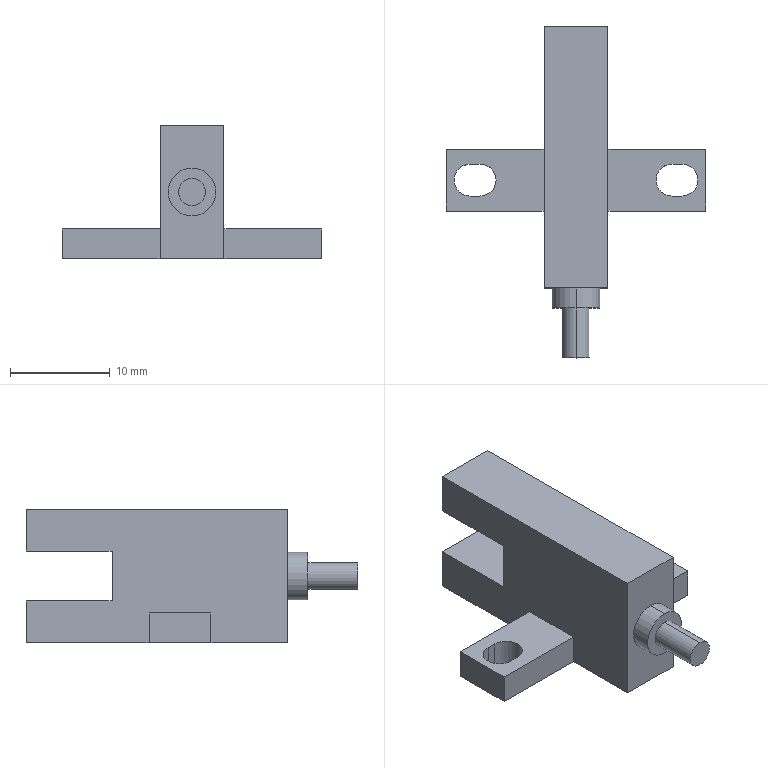Part | STEP file | 复件 aaPT-T44^复件 FFH85-PL-M75-B3-01_三轴模组 | 1 solid | 34 faces | box 26 x 33.2 x 13.4 mm | volume 2334 mm3 | plane 24 | cylinder 10 | commonest cylinder face diameters 3.2 x6 2.7 x2 4.8 x2
STEP:
#1=CARTESIAN_POINT('',(0.,-15.1,9.1));
#2=VERTEX_POINT('',#1);
#3=CARTESIAN_POINT('',(0.,-15.1,4.3));
#4=VERTEX_POINT('',#3);
#5=CARTESIAN_POINT('',(0.,-15.1,6.7));
#6=DIRECTION('',(0.,1.,0.));
#7=DIRECTION('',(0.,0.,1.));
#8=AXIS2_PLACEMENT_3D('',#5,#6,#7);
#9=CIRCLE('',#8,2.4);
#10=EDGE_CURVE('',#2,#4,#9,.T.);
#11=ORIENTED_EDGE('',*,*,#10,.T.);
#12=CARTESIAN_POINT('',(0.,-13.1,4.3));
#13=VERTEX_POINT('',#12);
#14=CARTESIAN_POINT('',(0.,-15.1,4.3));
#15=DIRECTION('',(0.,1.,0.));
#16=VECTOR('',#15,1000.);
#17=LINE('',#14,#16);
#18=EDGE_CURVE('',#4,#13,#17,.T.);
#19=ORIENTED_EDGE('',*,*,#18,.T.);
#20=CARTESIAN_POINT('',(0.,-13.1,9.1));
#21=VERTEX_POINT('',#20);
#22=CARTESIAN_POINT('',(0.,-13.1,6.7));
#23=DIRECTION('',(0.,-1.,0.));
#24=DIRECTION('',(0.,0.,1.));
#25=AXIS2_PLACEMENT_3D('',#22,#23,#24);
#26=CIRCLE('',#25,2.4);
#27=EDGE_CURVE('',#13,#21,#26,.T.);
#28=ORIENTED_EDGE('',*,*,#27,.T.);
#29=CARTESIAN_POINT('',(0.,-15.1,9.1));
#30=DIRECTION('',(0.,1.,0.));
#31=VECTOR('',#30,1000.);
#32=LINE('',#29,#31);
#33=EDGE_CURVE('',#2,#21,#32,.T.);
#34=ORIENTED_EDGE('',*,*,#33,.F.);
#35=EDGE_LOOP('',(#11,#19,#28,#34));
#36=FACE_OUTER_BOUND('',#35,.T.);
#37=CARTESIAN_POINT('',(0.,-15.1,6.7));
#38=DIRECTION('',(0.,1.,0.));
#39=DIRECTION('',(0.,0.,1.));
#40=AXIS2_PLACEMENT_3D('',#37,#38,#39);
#41=CYLINDRICAL_SURFACE('',#40,2.4);
#42=ADVANCED_FACE('',(#36),#41,.T.);
#43=CARTESIAN_POINT('',(12.2,-2.3,0.));
#44=VERTEX_POINT('',#43);
#45=CARTESIAN_POINT('',(10.575,-0.7002,0.));
#46=VERTEX_POINT('',#45);
#47=CARTESIAN_POINT('',(10.6,-2.3,0.));
#48=DIRECTION('',(0.,0.,1.));
#49=DIRECTION('',(1.,0.,0.));
#50=AXIS2_PLACEMENT_3D('',#47,#48,#49);
#51=CIRCLE('',#50,1.6);
#52=EDGE_CURVE('',#44,#46,#51,.T.);
#53=ORIENTED_EDGE('',*,*,#52,.F.);
#54=CARTESIAN_POINT('',(12.2,-2.3,3.));
#55=VERTEX_POINT('',#54);
#56=CARTESIAN_POINT('',(12.2,-2.3,0.));
#57=DIRECTION('',(0.,0.,1.));
#58=VECTOR('',#57,1000.);
#59=LINE('',#56,#58);
#60=EDGE_CURVE('',#44,#55,#59,.T.);
#61=ORIENTED_EDGE('',*,*,#60,.T.);
#62=CARTESIAN_POINT('',(10.575,-0.7002,3.));
#63=VERTEX_POINT('',#62);
#64=CARTESIAN_POINT('',(10.6,-2.3,3.));
#65=DIRECTION('',(0.,0.,1.));
#66=DIRECTION('',(1.,0.,0.));
#67=AXIS2_PLACEMENT_3D('',#64,#65,#66);
#68=CIRCLE('',#67,1.6);
#69=EDGE_CURVE('',#55,#63,#68,.T.);
#70=ORIENTED_EDGE('',*,*,#69,.T.);
#71=CARTESIAN_POINT('',(10.575,-0.7002,0.));
#72=DIRECTION('',(0.,0.,1.));
#73=VECTOR('',#72,1000.);
#74=LINE('',#71,#73);
#75=EDGE_CURVE('',#46,#63,#74,.T.);
#76=ORIENTED_EDGE('',*,*,#75,.F.);
#77=EDGE_LOOP('',(#53,#61,#70,#76));
#78=FACE_OUTER_BOUND('',#77,.T.);
#79=CARTESIAN_POINT('',(10.6,-2.3,0.));
#80=DIRECTION('',(0.,0.,1.));
#81=DIRECTION('',(1.,0.,0.));
#82=AXIS2_PLACEMENT_3D('',#79,#80,#81);
#83=CYLINDRICAL_SURFACE('',#82,1.6);
#84=ADVANCED_FACE('',(#78),#83,.F.);
#85=CARTESIAN_POINT('',(-8.,-2.3,0.));
#86=VERTEX_POINT('',#85);
#87=CARTESIAN_POINT('',(-9.6,-0.7002,0.));
#88=VERTEX_POINT('',#87);
#89=CARTESIAN_POINT('',(-9.6,-2.3,0.));
#90=DIRECTION('',(0.,0.,1.));
#91=DIRECTION('',(1.,0.,0.));
#92=AXIS2_PLACEMENT_3D('',#89,#90,#91);
#93=CIRCLE('',#92,1.6);
#94=EDGE_CURVE('',#86,#88,#93,.T.);
#95=ORIENTED_EDGE('',*,*,#94,.F.);
#96=CARTESIAN_POINT('',(-8.,-2.3,3.));
#97=VERTEX_POINT('',#96);
#98=CARTESIAN_POINT('',(-8.,-2.3,0.));
#99=DIRECTION('',(0.,0.,1.));
#100=VECTOR('',#99,1000.);
#101=LINE('',#98,#100);
#102=EDGE_CURVE('',#86,#97,#101,.T.);
#103=ORIENTED_EDGE('',*,*,#102,.T.);
#104=CARTESIAN_POINT('',(-9.6,-0.7002,3.));
#105=VERTEX_POINT('',#104);
#106=CARTESIAN_POINT('',(-9.6,-2.3,3.));
#107=DIRECTION('',(0.,0.,-1.));
#108=DIRECTION('',(1.,0.,0.));
#109=AXIS2_PLACEMENT_3D('',#106,#107,#108);
#110=CIRCLE('',#109,1.6);
#111=EDGE_CURVE('',#105,#97,#110,.T.);
#112=ORIENTED_EDGE('',*,*,#111,.F.);
#113=CARTESIAN_POINT('',(-9.6,-0.7002,0.));
#114=DIRECTION('',(0.,0.,1.));
#115=VECTOR('',#114,1000.);
#116=LINE('',#113,#115);
#117=EDGE_CURVE('',#88,#105,#116,.T.);
#118=ORIENTED_EDGE('',*,*,#117,.F.);
#119=EDGE_LOOP('',(#95,#103,#112,#118));
#120=FACE_OUTER_BOUND('',#119,.T.);
#121=CARTESIAN_POINT('',(-9.6,-2.3,0.));
#122=DIRECTION('',(0.,0.,1.));
#123=DIRECTION('',(1.,0.,0.));
#124=AXIS2_PLACEMENT_3D('',#121,#122,#123);
#125=CYLINDRICAL_SURFACE('',#124,1.6);
#126=ADVANCED_FACE('',(#120),#125,.F.);
#127=CARTESIAN_POINT('',(0.,-20.1,8.05));
#128=VERTEX_POINT('',#127);
#129=CARTESIAN_POINT('',(0.,-20.1,5.35));
#130=VERTEX_POINT('',#129);
#131=CARTESIAN_POINT('',(0.,-20.1,6.7));
#132=DIRECTION('',(0.,1.,0.));
#133=DIRECTION('',(0.,0.,1.));
#134=AXIS2_PLACEMENT_3D('',#131,#132,#133);
#135=CIRCLE('',#134,1.35);
#136=EDGE_CURVE('',#128,#130,#135,.T.);
#137=ORIENTED_EDGE('',*,*,#136,.T.);
#138=CARTESIAN_POINT('',(0.,-15.1,5.35));
#139=VERTEX_POINT('',#138);
#140=CARTESIAN_POINT('',(0.,-20.1,5.35));
#141=DIRECTION('',(0.,1.,0.));
#142=VECTOR('',#141,1000.);
#143=LINE('',#140,#142);
#144=EDGE_CURVE('',#130,#139,#143,.T.);
#145=ORIENTED_EDGE('',*,*,#144,.T.);
#146=CARTESIAN_POINT('',(0.,-15.1,8.05));
#147=VERTEX_POINT('',#146);
#148=CARTESIAN_POINT('',(0.,-15.1,6.7));
#149=DIRECTION('',(0.,1.,0.));
#150=DIRECTION('',(0.,0.,1.));
#151=AXIS2_PLACEMENT_3D('',#148,#149,#150);
#152=CIRCLE('',#151,1.35);
#153=EDGE_CURVE('',#147,#139,#152,.T.);
#154=ORIENTED_EDGE('',*,*,#153,.F.);
#155=CARTESIAN_POINT('',(0.,-20.1,8.05));
#156=DIRECTION('',(0.,1.,0.));
#157=VECTOR('',#156,1000.);
#158=LINE('',#155,#157);
#159=EDGE_CURVE('',#128,#147,#158,.T.);
#160=ORIENTED_EDGE('',*,*,#159,.F.);
#161=EDGE_LOOP('',(#137,#145,#154,#160));
#162=FACE_OUTER_BOUND('',#161,.T.);
#163=CARTESIAN_POINT('',(0.,-20.1,6.7));
#164=DIRECTION('',(0.,1.,0.));
#165=DIRECTION('',(0.,0.,1.));
#166=AXIS2_PLACEMENT_3D('',#163,#164,#165);
#167=CYLINDRICAL_SURFACE('',#166,1.35);
#168=ADVANCED_FACE('',(#162),#167,.T.);
#169=CARTESIAN_POINT('',(3.2,-13.1,0.));
#170=VERTEX_POINT('',#169);
#171=CARTESIAN_POINT('',(3.2,-13.1,13.4));
#172=VERTEX_POINT('',#171);
#173=CARTESIAN_POINT('',(3.2,-13.1,13.4));
#174=DIRECTION('',(0.,0.,1.));
#175=VECTOR('',#174,1000.);
#176=LINE('',#173,#175);
#177=EDGE_CURVE('',#170,#172,#176,.T.);
#178=ORIENTED_EDGE('',*,*,#177,.F.);
#179=CARTESIAN_POINT('',(3.2,-5.4,0.));
#180=VERTEX_POINT('',#179);
#181=CARTESIAN_POINT('',(3.2,-13.1,0.));
#182=DIRECTION('',(0.,-1.,0.));
#183=VECTOR('',#182,1000.);
#184=LINE('',#181,#183);
#185=EDGE_CURVE('',#180,#170,#184,.T.);
#186=ORIENTED_EDGE('',*,*,#185,.F.);
#187=CARTESIAN_POINT('',(3.2,-5.4,3.));
#188=VERTEX_POINT('',#187);
#189=CARTESIAN_POINT('',(3.2,-5.4,13.4));
#190=DIRECTION('',(0.,0.,-1.));
#191=VECTOR('',#190,1000.);
#192=LINE('',#189,#191);
#193=EDGE_CURVE('',#188,#180,#192,.T.);
#194=ORIENTED_EDGE('',*,*,#193,.F.);
#195=CARTESIAN_POINT('',(3.2,0.8,3.));
#196=VERTEX_POINT('',#195);
#197=CARTESIAN_POINT('',(3.2,-13.1,3.));
#198=DIRECTION('',(0.,-1.,0.));
#199=VECTOR('',#198,1000.);
#200=LINE('',#197,#199);
#201=EDGE_CURVE('',#196,#188,#200,.T.);
#202=ORIENTED_EDGE('',*,*,#201,.F.);
#203=CARTESIAN_POINT('',(3.2,0.8,0.));
#204=VERTEX_POINT('',#203);
#205=CARTESIAN_POINT('',(3.2,0.8,13.4));
#206=DIRECTION('',(0.,0.,1.));
#207=VECTOR('',#206,1000.);
#208=LINE('',#205,#207);
#209=EDGE_CURVE('',#204,#196,#208,.T.);
#210=ORIENTED_EDGE('',*,*,#209,.F.);
#211=CARTESIAN_POINT('',(3.2,13.1,0.));
#212=VERTEX_POINT('',#211);
#213=CARTESIAN_POINT('',(3.2,-13.1,0.));
#214=DIRECTION('',(0.,-1.,0.));
#215=VECTOR('',#214,1000.);
#216=LINE('',#213,#215);
#217=EDGE_CURVE('',#212,#204,#216,.T.);
#218=ORIENTED_EDGE('',*,*,#217,.F.);
#219=CARTESIAN_POINT('',(3.2,13.1,4.2));
#220=VERTEX_POINT('',#219);
#221=CARTESIAN_POINT('',(3.2,13.1,13.4));
#222=DIRECTION('',(0.,0.,-1.));
#223=VECTOR('',#222,1000.);
#224=LINE('',#221,#223);
#225=EDGE_CURVE('',#220,#212,#224,.T.);
#226=ORIENTED_EDGE('',*,*,#225,.F.);
#227=CARTESIAN_POINT('',(3.2,4.5,4.2));
#228=VERTEX_POINT('',#227);
#229=CARTESIAN_POINT('',(3.2,-13.1,4.2));
#230=DIRECTION('',(0.,1.,0.));
#231=VECTOR('',#230,1000.);
#232=LINE('',#229,#231);
#233=EDGE_CURVE('',#228,#220,#232,.T.);
#234=ORIENTED_EDGE('',*,*,#233,.F.);
#235=CARTESIAN_POINT('',(3.2,4.5,9.2));
#236=VERTEX_POINT('',#235);
#237=CARTESIAN_POINT('',(3.2,4.5,13.4));
#238=DIRECTION('',(0.,0.,-1.));
#239=VECTOR('',#238,1000.);
#240=LINE('',#237,#239);
#241=EDGE_CURVE('',#236,#228,#240,.T.);
#242=ORIENTED_EDGE('',*,*,#241,.F.);
#243=CARTESIAN_POINT('',(3.2,13.1,9.2));
#244=VERTEX_POINT('',#243);
#245=CARTESIAN_POINT('',(3.2,-13.1,9.2));
#246=DIRECTION('',(0.,-1.,0.));
#247=VECTOR('',#246,1000.);
#248=LINE('',#245,#247);
#249=EDGE_CURVE('',#244,#236,#248,.T.);
#250=ORIENTED_EDGE('',*,*,#249,.F.);
#251=CARTESIAN_POINT('',(3.2,13.1,13.4));
#252=VERTEX_POINT('',#251);
#253=CARTESIAN_POINT('',(3.2,13.1,13.4));
#254=DIRECTION('',(0.,0.,-1.));
#255=VECTOR('',#254,1000.);
#256=LINE('',#253,#255);
#257=EDGE_CURVE('',#252,#244,#256,.T.);
#258=ORIENTED_EDGE('',*,*,#257,.F.);
#259=CARTESIAN_POINT('',(3.2,-13.1,13.4));
#260=DIRECTION('',(0.,1.,0.));
#261=VECTOR('',#260,1000.);
#262=LINE('',#259,#261);
#263=EDGE_CURVE('',#172,#252,#262,.T.);
#264=ORIENTED_EDGE('',*,*,#263,.F.);
#265=EDGE_LOOP('',(#178,#186,#194,#202,#210,#218,#226,#234,#242,#250,#258,#264));
#266=FACE_OUTER_BOUND('',#265,.T.);
#267=CARTESIAN_POINT('',(3.2,-13.1,13.4));
#268=DIRECTION('',(-1.,0.,0.));
#269=DIRECTION('',(0.,0.,1.));
#270=AXIS2_PLACEMENT_3D('',#267,#268,#269);
#271=PLANE('',#270);
#272=ADVANCED_FACE('',(#266),#271,.F.);
#273=CARTESIAN_POINT('',(-3.2,13.1,13.4));
#274=VERTEX_POINT('',#273);
#275=CARTESIAN_POINT('',(13.,13.1,13.4));
#276=DIRECTION('',(1.,0.,0.));
#277=VECTOR('',#276,1000.);
#278=LINE('',#275,#277);
#279=EDGE_CURVE('',#274,#252,#278,.T.);
#280=ORIENTED_EDGE('',*,*,#279,.F.);
#281=CARTESIAN_POINT('',(-3.2,-13.1,13.4));
#282=VERTEX_POINT('',#281);
#283=CARTESIAN_POINT('',(-3.2,13.1,13.4));
#284=DIRECTION('',(0.,1.,0.));
#285=VECTOR('',#284,1000.);
#286=LINE('',#283,#285);
#287=EDGE_CURVE('',#282,#274,#286,.T.);
#288=ORIENTED_EDGE('',*,*,#287,.F.);
#289=CARTESIAN_POINT('',(13.,-13.1,13.4));
#290=DIRECTION('',(-1.,0.,0.));
#291=VECTOR('',#290,1000.);
#292=LINE('',#289,#291);
#293=EDGE_CURVE('',#172,#282,#292,.T.);
#294=ORIENTED_EDGE('',*,*,#293,.F.);
#295=ORIENTED_EDGE('',*,*,#263,.T.);
#296=EDGE_LOOP('',(#280,#288,#294,#295));
#297=FACE_OUTER_BOUND('',#296,.T.);
#298=CARTESIAN_POINT('',(13.,13.1,13.4));
#299=DIRECTION('',(0.,0.,-1.));
#300=DIRECTION('',(-1.,0.,0.));
#301=AXIS2_PLACEMENT_3D('',#298,#299,#300);
#302=PLANE('',#301);
#303=ADVANCED_FACE('',(#297),#302,.F.);
#304=ORIENTED_EDGE('',*,*,#293,.T.);
#305=CARTESIAN_POINT('',(-3.2,-13.1,0.));
#306=VERTEX_POINT('',#305);
#307=CARTESIAN_POINT('',(-3.2,-13.1,13.4));
#308=DIRECTION('',(0.,0.,1.));
#309=VECTOR('',#308,1000.);
#310=LINE('',#307,#309);
#311=EDGE_CURVE('',#306,#282,#310,.T.);
#312=ORIENTED_EDGE('',*,*,#311,.F.);
#313=CARTESIAN_POINT('',(-13.,-13.1,0.));
#314=DIRECTION('',(-1.,0.,0.));
#315=VECTOR('',#314,1000.);
#316=LINE('',#313,#315);
#317=EDGE_CURVE('',#170,#306,#316,.T.);
#318=ORIENTED_EDGE('',*,*,#317,.F.);
#319=ORIENTED_EDGE('',*,*,#177,.T.);
#320=EDGE_LOOP('',(#304,#312,#318,#319));
#321=FACE_OUTER_BOUND('',#320,.T.);
#322=CARTESIAN_POINT('',(0.,-13.1,6.7));
#323=DIRECTION('',(0.,-1.,0.));
#324=DIRECTION('',(0.,0.,1.));
#325=AXIS2_PLACEMENT_3D('',#322,#323,#324);
#326=CIRCLE('',#325,2.4);
#327=EDGE_CURVE('',#21,#13,#326,.T.);
#328=ORIENTED_EDGE('',*,*,#327,.F.);
#329=ORIENTED_EDGE('',*,*,#27,.F.);
#330=EDGE_LOOP('',(#328,#329));
#331=FACE_BOUND('',#330,.T.);
#332=CARTESIAN_POINT('',(-13.,-13.1,13.4));
#333=DIRECTION('',(0.,1.,0.));
#334=DIRECTION('',(0.,0.,1.));
#335=AXIS2_PLACEMENT_3D('',#332,#333,#334);
#336=PLANE('',#335);
#337=ADVANCED_FACE('',(#321,#331),#336,.F.);
#338=CARTESIAN_POINT('',(10.6,-3.9,0.));
#339=VERTEX_POINT('',#338);
#340=CARTESIAN_POINT('',(10.6,-2.3,0.));
#341=DIRECTION('',(0.,0.,1.));
#342=DIRECTION('',(1.,0.,0.));
#343=AXIS2_PLACEMENT_3D('',#340,#341,#342);
#344=CIRCLE('',#343,1.6);
#345=EDGE_CURVE('',#339,#44,#344,.T.);
#346=ORIENTED_EDGE('',*,*,#345,.T.);
#347=ORIENTED_EDGE('',*,*,#52,.T.);
#348=CARTESIAN_POINT('',(9.6,-0.7002,0.));
#349=VERTEX_POINT('',#348);
#350=CARTESIAN_POINT('',(10.575,-0.7002,0.));
#351=DIRECTION('',(-1.,0.,0.));
#352=VECTOR('',#351,1000.);
#353=LINE('',#350,#352);
#354=EDGE_CURVE('',#46,#349,#353,.T.);
#355=ORIENTED_EDGE('',*,*,#354,.T.);
#356=CARTESIAN_POINT('',(9.625,-3.9,0.));
#357=VERTEX_POINT('',#356);
#358=CARTESIAN_POINT('',(9.6,-2.3,0.));
#359=DIRECTION('',(0.,0.,1.));
#360=DIRECTION('',(1.,0.,0.));
#361=AXIS2_PLACEMENT_3D('',#358,#359,#360);
#362=CIRCLE('',#361,1.6);
#363=EDGE_CURVE('',#349,#357,#362,.T.);
#364=ORIENTED_EDGE('',*,*,#363,.T.);
#365=CARTESIAN_POINT('',(10.6,-3.9,0.));
#366=DIRECTION('',(1.,0.,0.));
#367=VECTOR('',#366,1000.);
#368=LINE('',#365,#367);
#369=EDGE_CURVE('',#357,#339,#368,.T.);
#370=ORIENTED_EDGE('',*,*,#369,.T.);
#371=EDGE_LOOP('',(#346,#347,#355,#364,#370));
#372=FACE_BOUND('',#371,.T.);
#373=CARTESIAN_POINT('',(-9.625,-3.9,0.));
#374=VERTEX_POINT('',#373);
#375=CARTESIAN_POINT('',(-9.6,-2.3,0.));
#376=DIRECTION('',(0.,0.,1.));
#377=DIRECTION('',(1.,0.,0.));
#378=AXIS2_PLACEMENT_3D('',#375,#376,#377);
#379=CIRCLE('',#378,1.6);
#380=EDGE_CURVE('',#374,#86,#379,.T.);
#381=ORIENTED_EDGE('',*,*,#380,.T.);
#382=ORIENTED_EDGE('',*,*,#94,.T.);
#383=CARTESIAN_POINT('',(-10.575,-0.7002,0.));
#384=VERTEX_POINT('',#383);
#385=CARTESIAN_POINT('',(-10.575,-0.7002,0.));
#386=DIRECTION('',(-1.,0.,0.));
#387=VECTOR('',#386,1000.);
#388=LINE('',#385,#387);
#389=EDGE_CURVE('',#88,#384,#388,.T.);
#390=ORIENTED_EDGE('',*,*,#389,.T.);
#391=CARTESIAN_POINT('',(-10.6,-3.9,0.));
#392=VERTEX_POINT('',#391);
#393=CARTESIAN_POINT('',(-10.6,-2.3,0.));
#394=DIRECTION('',(0.,0.,1.));
#395=DIRECTION('',(1.,0.,0.));
#396=AXIS2_PLACEMENT_3D('',#393,#394,#395);
#397=CIRCLE('',#396,1.6);
#398=EDGE_CURVE('',#384,#392,#397,.T.);
#399=ORIENTED_EDGE('',*,*,#398,.T.);
#400=CARTESIAN_POINT('',(-10.6,-3.9,0.));
#401=DIRECTION('',(1.,0.,0.));
#402=VECTOR('',#401,1000.);
#403=LINE('',#400,#402);
#404=EDGE_CURVE('',#392,#374,#403,.T.);
#405=ORIENTED_EDGE('',*,*,#404,.T.);
#406=EDGE_LOOP('',(#381,#382,#390,#399,#405));
#407=FACE_BOUND('',#406,.T.);
#408=CARTESIAN_POINT('',(-13.,0.8,0.));
#409=VERTEX_POINT('',#408);
#410=CARTESIAN_POINT('',(-3.2,0.8,0.));
#411=VERTEX_POINT('',#410);
#412=CARTESIAN_POINT('',(13.,0.8,0.));
#413=DIRECTION('',(1.,0.,0.));
#414=VECTOR('',#413,1000.);
#415=LINE('',#412,#414);
#416=EDGE_CURVE('',#409,#411,#415,.T.);
#417=ORIENTED_EDGE('',*,*,#416,.T.);
#418=CARTESIAN_POINT('',(-3.2,13.1,0.));
#419=VERTEX_POINT('',#418);
#420=CARTESIAN_POINT('',(-3.2,13.1,0.));
#421=DIRECTION('',(0.,1.,0.));
#422=VECTOR('',#421,1000.);
#423=LINE('',#420,#422);
#424=EDGE_CURVE('',#411,#419,#423,.T.);
#425=ORIENTED_EDGE('',*,*,#424,.T.);
#426=CARTESIAN_POINT('',(13.,13.1,0.));
#427=DIRECTION('',(1.,0.,0.));
#428=VECTOR('',#427,1000.);
#429=LINE('',#426,#428);
#430=EDGE_CURVE('',#419,#212,#429,.T.);
#431=ORIENTED_EDGE('',*,*,#430,.T.);
#432=ORIENTED_EDGE('',*,*,#217,.T.);
#433=CARTESIAN_POINT('',(13.,0.8,0.));
#434=VERTEX_POINT('',#433);
#435=CARTESIAN_POINT('',(13.,0.8,0.));
#436=DIRECTION('',(1.,0.,0.));
#437=VECTOR('',#436,1000.);
#438=LINE('',#435,#437);
#439=EDGE_CURVE('',#204,#434,#438,.T.);
#440=ORIENTED_EDGE('',*,*,#439,.T.);
#441=CARTESIAN_POINT('',(13.,-5.4,0.));
#442=VERTEX_POINT('',#441);
#443=CARTESIAN_POINT('',(13.,13.1,0.));
#444=DIRECTION('',(0.,-1.,0.));
#445=VECTOR('',#444,1000.);
#446=LINE('',#443,#445);
#447=EDGE_CURVE('',#434,#442,#446,.T.);
#448=ORIENTED_EDGE('',*,*,#447,.T.);
#449=CARTESIAN_POINT('',(13.,-5.4,0.));
#450=DIRECTION('',(-1.,0.,0.));
#451=VECTOR('',#450,1000.);
#452=LINE('',#449,#451);
#453=EDGE_CURVE('',#442,#180,#452,.T.);
#454=ORIENTED_EDGE('',*,*,#453,.T.);
#455=ORIENTED_EDGE('',*,*,#185,.T.);
#456=ORIENTED_EDGE('',*,*,#317,.T.);
#457=CARTESIAN_POINT('',(-3.2,-5.4,0.));
#458=VERTEX_POINT('',#457);
#459=CARTESIAN_POINT('',(-3.2,13.1,0.));
#460=DIRECTION('',(0.,1.,0.));
#461=VECTOR('',#460,1000.);
#462=LINE('',#459,#461);
#463=EDGE_CURVE('',#306,#458,#462,.T.);
#464=ORIENTED_EDGE('',*,*,#463,.T.);
#465=CARTESIAN_POINT('',(-13.,-5.4,0.));
#466=VERTEX_POINT('',#465);
#467=CARTESIAN_POINT('',(13.,-5.4,0.));
#468=DIRECTION('',(-1.,0.,0.));
#469=VECTOR('',#468,1000.);
#470=LINE('',#467,#469);
#471=EDGE_CURVE('',#458,#466,#470,.T.);
#472=ORIENTED_EDGE('',*,*,#471,.T.);
#473=CARTESIAN_POINT('',(-13.,13.1,0.));
#474=DIRECTION('',(0.,1.,0.));
#475=VECTOR('',#474,1000.);
#476=LINE('',#473,#475);
#477=EDGE_CURVE('',#466,#409,#476,.T.);
#478=ORIENTED_EDGE('',*,*,#477,.T.);
#479=EDGE_LOOP('',(#417,#425,#431,#432,#440,#448,#454,#455,#456,#464,#472,#478));
#480=FACE_OUTER_BOUND('',#479,.T.);
#481=CARTESIAN_POINT('',(13.,13.1,0.));
#482=DIRECTION('',(0.,0.,-1.));
#483=DIRECTION('',(-1.,0.,0.));
#484=AXIS2_PLACEMENT_3D('',#481,#482,#483);
#485=PLANE('',#484);
#486=ADVANCED_FACE('',(#372,#407,#480),#485,.T.);
#487=ORIENTED_EDGE('',*,*,#453,.F.);
#488=CARTESIAN_POINT('',(13.,-5.4,3.));
#489=VERTEX_POINT('',#488);
#490=CARTESIAN_POINT('',(13.,-5.4,0.));
#491=DIRECTION('',(0.,0.,-1.));
#492=VECTOR('',#491,1000.);
#493=LINE('',#490,#492);
#494=EDGE_CURVE('',#489,#442,#493,.T.);
#495=ORIENTED_EDGE('',*,*,#494,.F.);
#496=CARTESIAN_POINT('',(13.,-5.4,3.));
#497=DIRECTION('',(1.,0.,0.));
#498=VECTOR('',#497,1000.);
#499=LINE('',#496,#498);
#500=EDGE_CURVE('',#188,#489,#499,.T.);
#501=ORIENTED_EDGE('',*,*,#500,.F.);
#502=ORIENTED_EDGE('',*,*,#193,.T.);
#503=EDGE_LOOP('',(#487,#495,#501,#502));
#504=FACE_OUTER_BOUND('',#503,.T.);
#505=CARTESIAN_POINT('',(13.,-5.4,0.));
#506=DIRECTION('',(0.,1.,0.));
#507=DIRECTION('',(0.,0.,1.));
#508=AXIS2_PLACEMENT_3D('',#505,#506,#507);
#509=PLANE('',#508);
#510=ADVANCED_FACE('',(#504),#509,.F.);
#511=CARTESIAN_POINT('',(10.6,-3.9,3.));
#512=VERTEX_POINT('',#511);
#513=CARTESIAN_POINT('',(9.625,-3.9,3.));
#514=VERTEX_POINT('',#513);
#515=CARTESIAN_POINT('',(10.6,-3.9,3.));
#516=DIRECTION('',(-1.,0.,0.));
#517=VECTOR('',#516,1000.);
#518=LINE('',#515,#517);
#519=EDGE_CURVE('',#512,#514,#518,.T.);
#520=ORIENTED_EDGE('',*,*,#519,.T.);
#521=CARTESIAN_POINT('',(9.6,-0.7002,3.));
#522=VERTEX_POINT('',#521);
#523=CARTESIAN_POINT('',(9.6,-2.3,3.));
#524=DIRECTION('',(0.,0.,1.));
#525=DIRECTION('',(1.,0.,0.));
#526=AXIS2_PLACEMENT_3D('',#523,#524,#525);
#527=CIRCLE('',#526,1.6);
#528=EDGE_CURVE('',#522,#514,#527,.T.);
#529=ORIENTED_EDGE('',*,*,#528,.F.);
#530=CARTESIAN_POINT('',(10.575,-0.7002,3.));
#531=DIRECTION('',(1.,0.,0.));
#532=VECTOR('',#531,1000.);
#533=LINE('',#530,#532);
#534=EDGE_CURVE('',#522,#63,#533,.T.);
#535=ORIENTED_EDGE('',*,*,#534,.T.);
#536=ORIENTED_EDGE('',*,*,#69,.F.);
#537=CARTESIAN_POINT('',(10.6,-2.3,3.));
#538=DIRECTION('',(0.,0.,1.));
#539=DIRECTION('',(1.,0.,0.));
#540=AXIS2_PLACEMENT_3D('',#537,#538,#539);
#541=CIRCLE('',#540,1.6);
#542=EDGE_CURVE('',#512,#55,#541,.T.);
#543=ORIENTED_EDGE('',*,*,#542,.F.);
#544=EDGE_LOOP('',(#520,#529,#535,#536,#543));
#545=FACE_BOUND('',#544,.T.);
#546=ORIENTED_EDGE('',*,*,#201,.T.);
#547=ORIENTED_EDGE('',*,*,#500,.T.);
#548=CARTESIAN_POINT('',(13.,0.8,3.));
#549=VERTEX_POINT('',#548);
#550=CARTESIAN_POINT('',(13.,-13.1,3.));
#551=DIRECTION('',(0.,-1.,0.));
#552=VECTOR('',#551,1000.);
#553=LINE('',#550,#552);
#554=EDGE_CURVE('',#549,#489,#553,.T.);
#555=ORIENTED_EDGE('',*,*,#554,.F.);
#556=CARTESIAN_POINT('',(13.,0.8,3.));
#557=DIRECTION('',(1.,0.,0.));
#558=VECTOR('',#557,1000.);
#559=LINE('',#556,#558);
#560=EDGE_CURVE('',#196,#549,#559,.T.);
#561=ORIENTED_EDGE('',*,*,#560,.F.);
#562=EDGE_LOOP('',(#546,#547,#555,#561));
#563=FACE_OUTER_BOUND('',#562,.T.);
#564=CARTESIAN_POINT('',(13.,-13.1,3.));
#565=DIRECTION('',(0.,0.,-1.));
#566=DIRECTION('',(-1.,0.,0.));
#567=AXIS2_PLACEMENT_3D('',#564,#565,#566);
#568=PLANE('',#567);
#569=ADVANCED_FACE('',(#545,#563),#568,.F.);
#570=ORIENTED_EDGE('',*,*,#439,.F.);
#571=ORIENTED_EDGE('',*,*,#209,.T.);
#572=ORIENTED_EDGE('',*,*,#560,.T.);
#573=CARTESIAN_POINT('',(13.,0.8,0.));
#574=DIRECTION('',(0.,0.,1.));
#575=VECTOR('',#574,1000.);
#576=LINE('',#573,#575);
#577=EDGE_CURVE('',#434,#549,#576,.T.);
#578=ORIENTED_EDGE('',*,*,#577,.F.);
#579=EDGE_LOOP('',(#570,#571,#572,#578));
#580=FACE_OUTER_BOUND('',#579,.T.);
#581=CARTESIAN_POINT('',(13.,0.8,0.));
#582=DIRECTION('',(0.,-1.,0.));
#583=DIRECTION('',(0.,0.,-1.));
#584=AXIS2_PLACEMENT_3D('',#581,#582,#583);
#585=PLANE('',#584);
#586=ADVANCED_FACE('',(#580),#585,.F.);
#587=CARTESIAN_POINT('',(-3.2,13.1,4.2));
#588=VERTEX_POINT('',#587);
#589=CARTESIAN_POINT('',(-3.2,13.1,13.4));
#590=DIRECTION('',(0.,0.,-1.));
#591=VECTOR('',#590,1000.);
#592=LINE('',#589,#591);
#593=EDGE_CURVE('',#588,#419,#592,.T.);
#594=ORIENTED_EDGE('',*,*,#593,.F.);
#595=CARTESIAN_POINT('',(-13.,13.1,4.2));
#596=DIRECTION('',(-1.,0.,0.));
#597=VECTOR('',#596,1000.);
#598=LINE('',#595,#597);
#599=EDGE_CURVE('',#220,#588,#598,.T.);
#600=ORIENTED_EDGE('',*,*,#599,.F.);
#601=ORIENTED_EDGE('',*,*,#225,.T.);
#602=ORIENTED_EDGE('',*,*,#430,.F.);
#603=EDGE_LOOP('',(#594,#600,#601,#602));
#604=FACE_OUTER_BOUND('',#603,.T.);
#605=CARTESIAN_POINT('',(-13.,13.1,13.4));
#606=DIRECTION('',(0.,-1.,0.));
#607=DIRECTION('',(0.,0.,-1.));
#608=AXIS2_PLACEMENT_3D('',#605,#606,#607);
#609=PLANE('',#608);
#610=ADVANCED_FACE('',(#604),#609,.F.);
#611=ORIENTED_EDGE('',*,*,#599,.T.);
#612=CARTESIAN_POINT('',(-3.2,4.5,4.2));
#613=VERTEX_POINT('',#612);
#614=CARTESIAN_POINT('',(-3.2,13.1,4.2));
#615=DIRECTION('',(0.,1.,0.));
#616=VECTOR('',#615,1000.);
#617=LINE('',#614,#616);
#618=EDGE_CURVE('',#613,#588,#617,.T.);
#619=ORIENTED_EDGE('',*,*,#618,.F.);
#620=CARTESIAN_POINT('',(-13.,4.5,4.2));
#621=DIRECTION('',(-1.,0.,0.));
#622=VECTOR('',#621,1000.);
#623=LINE('',#620,#622);
#624=EDGE_CURVE('',#228,#613,#623,.T.);
#625=ORIENTED_EDGE('',*,*,#624,.F.);
#626=ORIENTED_EDGE('',*,*,#233,.T.);
#627=EDGE_LOOP('',(#611,#619,#625,#626));
#628=FACE_OUTER_BOUND('',#627,.T.);
#629=CARTESIAN_POINT('',(-13.,13.1,4.2));
#630=DIRECTION('',(0.,0.,-1.));
#631=DIRECTION('',(0.,1.,0.));
#632=AXIS2_PLACEMENT_3D('',#629,#630,#631);
#633=PLANE('',#632);
#634=ADVANCED_FACE('',(#628),#633,.F.);
#635=ORIENTED_EDGE('',*,*,#624,.T.);
#636=CARTESIAN_POINT('',(-3.2,4.5,9.2));
#637=VERTEX_POINT('',#636);
#638=CARTESIAN_POINT('',(-3.2,4.5,9.2));
#639=DIRECTION('',(0.,0.,-1.));
#640=VECTOR('',#639,1000.);
#641=LINE('',#638,#640);
#642=EDGE_CURVE('',#637,#613,#641,.T.);
#643=ORIENTED_EDGE('',*,*,#642,.F.);
#644=CARTESIAN_POINT('',(-13.,4.5,9.2));
#645=DIRECTION('',(-1.,0.,0.));
#646=VECTOR('',#645,1000.);
#647=LINE('',#644,#646);
#648=EDGE_CURVE('',#236,#637,#647,.T.);
#649=ORIENTED_EDGE('',*,*,#648,.F.);
#650=ORIENTED_EDGE('',*,*,#241,.T.);
#651=EDGE_LOOP('',(#635,#643,#649,#650));
#652=FACE_OUTER_BOUND('',#651,.T.);
#653=CARTESIAN_POINT('',(-13.,4.5,9.2));
#654=DIRECTION('',(0.,-1.,0.));
#655=DIRECTION('',(0.,0.,-1.));
#656=AXIS2_PLACEMENT_3D('',#653,#654,#655);
#657=PLANE('',#656);
#658=ADVANCED_FACE('',(#652),#657,.F.);
#659=ORIENTED_EDGE('',*,*,#648,.T.);
#660=CARTESIAN_POINT('',(-3.2,13.1,9.2));
#661=VERTEX_POINT('',#660);
#662=CARTESIAN_POINT('',(-3.2,13.1,9.2));
#663=DIRECTION('',(0.,-1.,0.));
#664=VECTOR('',#663,1000.);
#665=LINE('',#662,#664);
#666=EDGE_CURVE('',#661,#637,#665,.T.);
#667=ORIENTED_EDGE('',*,*,#666,.F.);
#668=CARTESIAN_POINT('',(-13.,13.1,9.2));
#669=DIRECTION('',(-1.,0.,0.));
#670=VECTOR('',#669,1000.);
#671=LINE('',#668,#670);
#672=EDGE_CURVE('',#244,#661,#671,.T.);
#673=ORIENTED_EDGE('',*,*,#672,.F.);
#674=ORIENTED_EDGE('',*,*,#249,.T.);
#675=EDGE_LOOP('',(#659,#667,#673,#674));
#676=FACE_OUTER_BOUND('',#675,.T.);
#677=CARTESIAN_POINT('',(-13.,13.1,9.2));
#678=DIRECTION('',(0.,0.,1.));
#679=DIRECTION('',(0.,-1.,0.));
#680=AXIS2_PLACEMENT_3D('',#677,#678,#679);
#681=PLANE('',#680);
#682=ADVANCED_FACE('',(#676),#681,.F.);
#683=ORIENTED_EDGE('',*,*,#672,.T.);
#684=CARTESIAN_POINT('',(-3.2,13.1,13.4));
#685=DIRECTION('',(0.,0.,-1.));
#686=VECTOR('',#685,1000.);
#687=LINE('',#684,#686);
#688=EDGE_CURVE('',#274,#661,#687,.T.);
#689=ORIENTED_EDGE('',*,*,#688,.F.);
#690=ORIENTED_EDGE('',*,*,#279,.T.);
#691=ORIENTED_EDGE('',*,*,#257,.T.);
#692=EDGE_LOOP('',(#683,#689,#690,#691));
#693=FACE_OUTER_BOUND('',#692,.T.);
#694=CARTESIAN_POINT('',(-13.,13.1,13.4));
#695=DIRECTION('',(0.,-1.,0.));
#696=DIRECTION('',(0.,0.,-1.));
#697=AXIS2_PLACEMENT_3D('',#694,#695,#696);
#698=PLANE('',#697);
#699=ADVANCED_FACE('',(#693),#698,.F.);
#700=ORIENTED_EDGE('',*,*,#593,.T.);
#701=ORIENTED_EDGE('',*,*,#424,.F.);
#702=CARTESIAN_POINT('',(-3.2,0.8,3.));
#703=VERTEX_POINT('',#702);
#704=CARTESIAN_POINT('',(-3.2,0.8,13.4));
#705=DIRECTION('',(0.,0.,-1.));
#706=VECTOR('',#705,1000.);
#707=LINE('',#704,#706);
#708=EDGE_CURVE('',#703,#411,#707,.T.);
#709=ORIENTED_EDGE('',*,*,#708,.F.);
#710=CARTESIAN_POINT('',(-3.2,-5.4,3.));
#711=VERTEX_POINT('',#710);
#712=CARTESIAN_POINT('',(-3.2,-13.1,3.));
#713=DIRECTION('',(0.,1.,0.));
#714=VECTOR('',#713,1000.);
#715=LINE('',#712,#714);
#716=EDGE_CURVE('',#711,#703,#715,.T.);
#717=ORIENTED_EDGE('',*,*,#716,.F.);
#718=CARTESIAN_POINT('',(-3.2,-5.4,13.4));
#719=DIRECTION('',(0.,0.,1.));
#720=VECTOR('',#719,1000.);
#721=LINE('',#718,#720);
#722=EDGE_CURVE('',#458,#711,#721,.T.);
#723=ORIENTED_EDGE('',*,*,#722,.F.);
#724=ORIENTED_EDGE('',*,*,#463,.F.);
#725=ORIENTED_EDGE('',*,*,#311,.T.);
#726=ORIENTED_EDGE('',*,*,#287,.T.);
#727=ORIENTED_EDGE('',*,*,#688,.T.);
#728=ORIENTED_EDGE('',*,*,#666,.T.);
#729=ORIENTED_EDGE('',*,*,#642,.T.);
#730=ORIENTED_EDGE('',*,*,#618,.T.);
#731=EDGE_LOOP('',(#700,#701,#709,#717,#723,#724,#725,#726,#727,#728,#729,#730));
#732=FACE_OUTER_BOUND('',#731,.T.);
#733=CARTESIAN_POINT('',(-3.2,-13.1,13.4));
#734=DIRECTION('',(1.,0.,0.));
#735=DIRECTION('',(0.,0.,-1.));
#736=AXIS2_PLACEMENT_3D('',#733,#734,#735);
#737=PLANE('',#736);
#738=ADVANCED_FACE('',(#732),#737,.F.);
#739=ORIENTED_EDGE('',*,*,#18,.F.);
#740=CARTESIAN_POINT('',(0.,-15.1,6.7));
#741=DIRECTION('',(0.,1.,0.));
#742=DIRECTION('',(0.,0.,1.));
#743=AXIS2_PLACEMENT_3D('',#740,#741,#742);
#744=CIRCLE('',#743,2.4);
#745=EDGE_CURVE('',#4,#2,#744,.T.);
#746=ORIENTED_EDGE('',*,*,#745,.T.);
#747=ORIENTED_EDGE('',*,*,#33,.T.);
#748=ORIENTED_EDGE('',*,*,#327,.T.);
#749=EDGE_LOOP('',(#739,#746,#747,#748));
#750=FACE_OUTER_BOUND('',#749,.T.);
#751=CARTESIAN_POINT('',(0.,-15.1,6.7));
#752=DIRECTION('',(0.,1.,0.));
#753=DIRECTION('',(0.,0.,1.));
#754=AXIS2_PLACEMENT_3D('',#751,#752,#753);
#755=CYLINDRICAL_SURFACE('',#754,2.4);
#756=ADVANCED_FACE('',(#750),#755,.T.);
#757=ORIENTED_EDGE('',*,*,#60,.F.);
#758=ORIENTED_EDGE('',*,*,#345,.F.);
#759=CARTESIAN_POINT('',(10.6,-3.9,0.));
#760=DIRECTION('',(0.,0.,-1.));
#761=VECTOR('',#760,1000.);
#762=LINE('',#759,#761);
#763=EDGE_CURVE('',#512,#339,#762,.T.);
#764=ORIENTED_EDGE('',*,*,#763,.F.);
#765=ORIENTED_EDGE('',*,*,#542,.T.);
#766=EDGE_LOOP('',(#757,#758,#764,#765));
#767=FACE_OUTER_BOUND('',#766,.T.);
#768=CARTESIAN_POINT('',(10.6,-2.3,0.));
#769=DIRECTION('',(0.,0.,1.));
#770=DIRECTION('',(1.,0.,0.));
#771=AXIS2_PLACEMENT_3D('',#768,#769,#770);
#772=CYLINDRICAL_SURFACE('',#771,1.6);
#773=ADVANCED_FACE('',(#767),#772,.F.);
#774=ORIENTED_EDGE('',*,*,#363,.F.);
#775=CARTESIAN_POINT('',(9.6,-0.7002,0.));
#776=DIRECTION('',(0.,0.,-1.));
#777=VECTOR('',#776,1000.);
#778=LINE('',#775,#777);
#779=EDGE_CURVE('',#522,#349,#778,.T.);
#780=ORIENTED_EDGE('',*,*,#779,.F.);
#781=ORIENTED_EDGE('',*,*,#528,.T.);
#782=CARTESIAN_POINT('',(9.625,-3.9,0.));
#783=DIRECTION('',(0.,0.,1.));
#784=VECTOR('',#783,1000.);
#785=LINE('',#782,#784);
#786=EDGE_CURVE('',#357,#514,#785,.T.);
#787=ORIENTED_EDGE('',*,*,#786,.F.);
#788=EDGE_LOOP('',(#774,#780,#781,#787));
#789=FACE_OUTER_BOUND('',#788,.T.);
#790=CARTESIAN_POINT('',(9.6,-2.3,0.));
#791=DIRECTION('',(0.,0.,1.));
#792=DIRECTION('',(1.,0.,0.));
#793=AXIS2_PLACEMENT_3D('',#790,#791,#792);
#794=CYLINDRICAL_SURFACE('',#793,1.6);
#795=ADVANCED_FACE('',(#789),#794,.F.);
#796=ORIENTED_EDGE('',*,*,#102,.F.);
#797=ORIENTED_EDGE('',*,*,#380,.F.);
#798=CARTESIAN_POINT('',(-9.625,-3.9,3.));
#799=VERTEX_POINT('',#798);
#800=CARTESIAN_POINT('',(-9.625,-3.9,0.));
#801=DIRECTION('',(0.,0.,-1.));
#802=VECTOR('',#801,1000.);
#803=LINE('',#800,#802);
#804=EDGE_CURVE('',#799,#374,#803,.T.);
#805=ORIENTED_EDGE('',*,*,#804,.F.);
#806=CARTESIAN_POINT('',(-9.6,-2.3,3.));
#807=DIRECTION('',(0.,0.,-1.));
#808=DIRECTION('',(1.,0.,0.));
#809=AXIS2_PLACEMENT_3D('',#806,#807,#808);
#810=CIRCLE('',#809,1.6);
#811=EDGE_CURVE('',#97,#799,#810,.T.);
#812=ORIENTED_EDGE('',*,*,#811,.F.);
#813=EDGE_LOOP('',(#796,#797,#805,#812));
#814=FACE_OUTER_BOUND('',#813,.T.);
#815=CARTESIAN_POINT('',(-9.6,-2.3,0.));
#816=DIRECTION('',(0.,0.,1.));
#817=DIRECTION('',(1.,0.,0.));
#818=AXIS2_PLACEMENT_3D('',#815,#816,#817);
#819=CYLINDRICAL_SURFACE('',#818,1.6);
#820=ADVANCED_FACE('',(#814),#819,.F.);
#821=ORIENTED_EDGE('',*,*,#398,.F.);
#822=CARTESIAN_POINT('',(-10.575,-0.7002,3.));
#823=VERTEX_POINT('',#822);
#824=CARTESIAN_POINT('',(-10.575,-0.7002,0.));
#825=DIRECTION('',(0.,0.,-1.));
#826=VECTOR('',#825,1000.);
#827=LINE('',#824,#826);
#828=EDGE_CURVE('',#823,#384,#827,.T.);
#829=ORIENTED_EDGE('',*,*,#828,.F.);
#830=CARTESIAN_POINT('',(-10.6,-3.9,3.));
#831=VERTEX_POINT('',#830);
#832=CARTESIAN_POINT('',(-10.6,-2.3,3.));
#833=DIRECTION('',(0.,0.,-1.));
#834=DIRECTION('',(1.,0.,0.));
#835=AXIS2_PLACEMENT_3D('',#832,#833,#834);
#836=CIRCLE('',#835,1.6);
#837=EDGE_CURVE('',#831,#823,#836,.T.);
#838=ORIENTED_EDGE('',*,*,#837,.F.);
#839=CARTESIAN_POINT('',(-10.6,-3.9,0.));
#840=DIRECTION('',(0.,0.,1.));
#841=VECTOR('',#840,1000.);
#842=LINE('',#839,#841);
#843=EDGE_CURVE('',#392,#831,#842,.T.);
#844=ORIENTED_EDGE('',*,*,#843,.F.);
#845=EDGE_LOOP('',(#821,#829,#838,#844));
#846=FACE_OUTER_BOUND('',#845,.T.);
#847=CARTESIAN_POINT('',(-10.6,-2.3,0.));
#848=DIRECTION('',(0.,0.,1.));
#849=DIRECTION('',(1.,0.,0.));
#850=AXIS2_PLACEMENT_3D('',#847,#848,#849);
#851=CYLINDRICAL_SURFACE('',#850,1.6);
#852=ADVANCED_FACE('',(#846),#851,.F.);
#853=ORIENTED_EDGE('',*,*,#416,.F.);
#854=CARTESIAN_POINT('',(-13.,0.8,3.));
#855=VERTEX_POINT('',#854);
#856=CARTESIAN_POINT('',(-13.,0.8,0.));
#857=DIRECTION('',(0.,0.,-1.));
#858=VECTOR('',#857,1000.);
#859=LINE('',#856,#858);
#860=EDGE_CURVE('',#855,#409,#859,.T.);
#861=ORIENTED_EDGE('',*,*,#860,.F.);
#862=CARTESIAN_POINT('',(-13.,0.8,3.));
#863=DIRECTION('',(-1.,0.,0.));
#864=VECTOR('',#863,1000.);
#865=LINE('',#862,#864);
#866=EDGE_CURVE('',#703,#855,#865,.T.);
#867=ORIENTED_EDGE('',*,*,#866,.F.);
#868=ORIENTED_EDGE('',*,*,#708,.T.);
#869=EDGE_LOOP('',(#853,#861,#867,#868));
#870=FACE_OUTER_BOUND('',#869,.T.);
#871=CARTESIAN_POINT('',(-13.,0.8,0.));
#872=DIRECTION('',(0.,-1.,0.));
#873=DIRECTION('',(0.,0.,-1.));
#874=AXIS2_PLACEMENT_3D('',#871,#872,#873);
#875=PLANE('',#874);
#876=ADVANCED_FACE('',(#870),#875,.F.);
#877=CARTESIAN_POINT('',(-13.,-5.4,3.));
#878=VERTEX_POINT('',#877);
#879=CARTESIAN_POINT('',(-13.,-13.1,3.));
#880=DIRECTION('',(0.,-1.,0.));
#881=VECTOR('',#880,1000.);
#882=LINE('',#879,#881);
#883=EDGE_CURVE('',#855,#878,#882,.T.);
#884=ORIENTED_EDGE('',*,*,#883,.F.);
#885=ORIENTED_EDGE('',*,*,#860,.T.);
#886=ORIENTED_EDGE('',*,*,#477,.F.);
#887=CARTESIAN_POINT('',(-13.,-5.4,13.4));
#888=DIRECTION('',(0.,0.,-1.));
#889=VECTOR('',#888,1000.);
#890=LINE('',#887,#889);
#891=EDGE_CURVE('',#878,#466,#890,.T.);
#892=ORIENTED_EDGE('',*,*,#891,.F.);
#893=EDGE_LOOP('',(#884,#885,#886,#892));
#894=FACE_OUTER_BOUND('',#893,.T.);
#895=CARTESIAN_POINT('',(-13.,-13.1,13.4));
#896=DIRECTION('',(1.,0.,0.));
#897=DIRECTION('',(0.,0.,-1.));
#898=AXIS2_PLACEMENT_3D('',#895,#896,#897);
#899=PLANE('',#898);
#900=ADVANCED_FACE('',(#894),#899,.F.);
#901=ORIENTED_EDGE('',*,*,#471,.F.);
#902=ORIENTED_EDGE('',*,*,#722,.T.);
#903=CARTESIAN_POINT('',(-13.,-5.4,3.));
#904=DIRECTION('',(1.,0.,0.));
#905=VECTOR('',#904,1000.);
#906=LINE('',#903,#905);
#907=EDGE_CURVE('',#878,#711,#906,.T.);
#908=ORIENTED_EDGE('',*,*,#907,.F.);
#909=ORIENTED_EDGE('',*,*,#891,.T.);
#910=EDGE_LOOP('',(#901,#902,#908,#909));
#911=FACE_OUTER_BOUND('',#910,.T.);
#912=CARTESIAN_POINT('',(-13.,-5.4,0.));
#913=DIRECTION('',(0.,1.,0.));
#914=DIRECTION('',(0.,0.,1.));
#915=AXIS2_PLACEMENT_3D('',#912,#913,#914);
#916=PLANE('',#915);
#917=ADVANCED_FACE('',(#911),#916,.F.);
#918=ORIENTED_EDGE('',*,*,#554,.T.);
#919=ORIENTED_EDGE('',*,*,#494,.T.);
#920=ORIENTED_EDGE('',*,*,#447,.F.);
#921=ORIENTED_EDGE('',*,*,#577,.T.);
#922=EDGE_LOOP('',(#918,#919,#920,#921));
#923=FACE_OUTER_BOUND('',#922,.T.);
#924=CARTESIAN_POINT('',(13.,-13.1,13.4));
#925=DIRECTION('',(-1.,0.,0.));
#926=DIRECTION('',(0.,0.,1.));
#927=AXIS2_PLACEMENT_3D('',#924,#925,#926);
#928=PLANE('',#927);
#929=ADVANCED_FACE('',(#923),#928,.F.);
#930=ORIENTED_EDGE('',*,*,#111,.T.);
#931=ORIENTED_EDGE('',*,*,#811,.T.);
#932=CARTESIAN_POINT('',(-13.,-3.9,3.));
#933=DIRECTION('',(1.,0.,0.));
#934=VECTOR('',#933,1000.);
#935=LINE('',#932,#934);
#936=EDGE_CURVE('',#831,#799,#935,.T.);
#937=ORIENTED_EDGE('',*,*,#936,.F.);
#938=ORIENTED_EDGE('',*,*,#837,.T.);
#939=CARTESIAN_POINT('',(-13.,-0.7002,3.));
#940=DIRECTION('',(-1.,0.,0.));
#941=VECTOR('',#940,1000.);
#942=LINE('',#939,#941);
#943=EDGE_CURVE('',#105,#823,#942,.T.);
#944=ORIENTED_EDGE('',*,*,#943,.F.);
#945=EDGE_LOOP('',(#930,#931,#937,#938,#944));
#946=FACE_BOUND('',#945,.T.);
#947=ORIENTED_EDGE('',*,*,#716,.T.);
#948=ORIENTED_EDGE('',*,*,#866,.T.);
#949=ORIENTED_EDGE('',*,*,#883,.T.);
#950=ORIENTED_EDGE('',*,*,#907,.T.);
#951=EDGE_LOOP('',(#947,#948,#949,#950));
#952=FACE_OUTER_BOUND('',#951,.T.);
#953=CARTESIAN_POINT('',(-13.,-13.1,3.));
#954=DIRECTION('',(0.,0.,-1.));
#955=DIRECTION('',(-1.,0.,0.));
#956=AXIS2_PLACEMENT_3D('',#953,#954,#955);
#957=PLANE('',#956);
#958=ADVANCED_FACE('',(#946,#952),#957,.F.);
#959=ORIENTED_EDGE('',*,*,#10,.F.);
#960=ORIENTED_EDGE('',*,*,#745,.F.);
#961=EDGE_LOOP('',(#959,#960));
#962=FACE_OUTER_BOUND('',#961,.T.);
#963=ORIENTED_EDGE('',*,*,#153,.T.);
#964=CARTESIAN_POINT('',(0.,-15.1,6.7));
#965=DIRECTION('',(0.,1.,0.));
#966=DIRECTION('',(0.,0.,1.));
#967=AXIS2_PLACEMENT_3D('',#964,#965,#966);
#968=CIRCLE('',#967,1.35);
#969=EDGE_CURVE('',#139,#147,#968,.T.);
#970=ORIENTED_EDGE('',*,*,#969,.T.);
#971=EDGE_LOOP('',(#963,#970));
#972=FACE_BOUND('',#971,.T.);
#973=CARTESIAN_POINT('',(0.,-15.1,6.7));
#974=DIRECTION('',(0.,-1.,0.));
#975=DIRECTION('',(0.,0.,-1.));
#976=AXIS2_PLACEMENT_3D('',#973,#974,#975);
#977=PLANE('',#976);
#978=ADVANCED_FACE('',(#962,#972),#977,.T.);
#979=ORIENTED_EDGE('',*,*,#354,.F.);
#980=ORIENTED_EDGE('',*,*,#75,.T.);
#981=ORIENTED_EDGE('',*,*,#534,.F.);
#982=ORIENTED_EDGE('',*,*,#779,.T.);
#983=EDGE_LOOP('',(#979,#980,#981,#982));
#984=FACE_OUTER_BOUND('',#983,.T.);
#985=CARTESIAN_POINT('',(10.575,-0.7002,0.));
#986=DIRECTION('',(0.,1.,0.));
#987=DIRECTION('',(0.,0.,1.));
#988=AXIS2_PLACEMENT_3D('',#985,#986,#987);
#989=PLANE('',#988);
#990=ADVANCED_FACE('',(#984),#989,.F.);
#991=ORIENTED_EDGE('',*,*,#369,.F.);
#992=ORIENTED_EDGE('',*,*,#786,.T.);
#993=ORIENTED_EDGE('',*,*,#519,.F.);
#994=ORIENTED_EDGE('',*,*,#763,.T.);
#995=EDGE_LOOP('',(#991,#992,#993,#994));
#996=FACE_OUTER_BOUND('',#995,.T.);
#997=CARTESIAN_POINT('',(10.6,-3.9,0.));
#998=DIRECTION('',(0.,-1.,0.));
#999=DIRECTION('',(1.,0.,0.));
#1000=AXIS2_PLACEMENT_3D('',#997,#998,#999);
#1001=PLANE('',#1000);
#1002=ADVANCED_FACE('',(#996),#1001,.F.);
#1003=ORIENTED_EDGE('',*,*,#389,.F.);
#1004=ORIENTED_EDGE('',*,*,#117,.T.);
#1005=ORIENTED_EDGE('',*,*,#943,.T.);
#1006=ORIENTED_EDGE('',*,*,#828,.T.);
#1007=EDGE_LOOP('',(#1003,#1004,#1005,#1006));
#1008=FACE_OUTER_BOUND('',#1007,.T.);
#1009=CARTESIAN_POINT('',(-10.575,-0.7002,0.));
#1010=DIRECTION('',(0.,1.,0.));
#1011=DIRECTION('',(-1.,0.,0.));
#1012=AXIS2_PLACEMENT_3D('',#1009,#1010,#1011);
#1013=PLANE('',#1012);
#1014=ADVANCED_FACE('',(#1008),#1013,.F.);
#1015=ORIENTED_EDGE('',*,*,#404,.F.);
#1016=ORIENTED_EDGE('',*,*,#843,.T.);
#1017=ORIENTED_EDGE('',*,*,#936,.T.);
#1018=ORIENTED_EDGE('',*,*,#804,.T.);
#1019=EDGE_LOOP('',(#1015,#1016,#1017,#1018));
#1020=FACE_OUTER_BOUND('',#1019,.T.);
#1021=CARTESIAN_POINT('',(-10.6,-3.9,0.));
#1022=DIRECTION('',(0.,-1.,0.));
#1023=DIRECTION('',(0.,0.,-1.));
#1024=AXIS2_PLACEMENT_3D('',#1021,#1022,#1023);
#1025=PLANE('',#1024);
#1026=ADVANCED_FACE('',(#1020),#1025,.F.);
#1027=ORIENTED_EDGE('',*,*,#144,.F.);
#1028=CARTESIAN_POINT('',(0.,-20.1,6.7));
#1029=DIRECTION('',(0.,1.,0.));
#1030=DIRECTION('',(0.,0.,1.));
#1031=AXIS2_PLACEMENT_3D('',#1028,#1029,#1030);
#1032=CIRCLE('',#1031,1.35);
#1033=EDGE_CURVE('',#130,#128,#1032,.T.);
#1034=ORIENTED_EDGE('',*,*,#1033,.T.);
#1035=ORIENTED_EDGE('',*,*,#159,.T.);
#1036=ORIENTED_EDGE('',*,*,#969,.F.);
#1037=EDGE_LOOP('',(#1027,#1034,#1035,#1036));
#1038=FACE_OUTER_BOUND('',#1037,.T.);
#1039=CARTESIAN_POINT('',(0.,-20.1,6.7));
#1040=DIRECTION('',(0.,1.,0.));
#1041=DIRECTION('',(0.,0.,1.));
#1042=AXIS2_PLACEMENT_3D('',#1039,#1040,#1041);
#1043=CYLINDRICAL_SURFACE('',#1042,1.35);
#1044=ADVANCED_FACE('',(#1038),#1043,.T.);
#1045=ORIENTED_EDGE('',*,*,#136,.F.);
#1046=ORIENTED_EDGE('',*,*,#1033,.F.);
#1047=EDGE_LOOP('',(#1045,#1046));
#1048=FACE_OUTER_BOUND('',#1047,.T.);
#1049=CARTESIAN_POINT('',(0.,-20.1,6.7));
#1050=DIRECTION('',(0.,-1.,0.));
#1051=DIRECTION('',(0.,0.,-1.));
#1052=AXIS2_PLACEMENT_3D('',#1049,#1050,#1051);
#1053=PLANE('',#1052);
#1054=ADVANCED_FACE('',(#1048),#1053,.T.);
#1055=CLOSED_SHELL('',(#42,#84,#126,#168,#272,#303,#337,#486,#510,#569,#586,#610,#634,#658,#682,#699,#738,#756,#773,#795,#820,#852,#876,#900,#917,#929,#958,#978,#990,#1002,#1014,#1026,#1044,#1054));
#1056=MANIFOLD_SOLID_BREP('',#1055);
#1057=CARTESIAN_POINT('',(0.,0.,0.));
#1058=DIRECTION('',(0.,0.,1.));
#1059=DIRECTION('',(1.,0.,0.));
#1060=AXIS2_PLACEMENT_3D('',#1057,#1058,#1059);
#1061=(LENGTH_UNIT()NAMED_UNIT(*)SI_UNIT(.MILLI.,.METRE.));
#1062=UNCERTAINTY_MEASURE_WITH_UNIT(LENGTH_MEASURE(0.00001),#1061,'','');
#1063=(NAMED_UNIT(*)PLANE_ANGLE_UNIT()SI_UNIT($,.RADIAN.));
#1064=(NAMED_UNIT(*)SI_UNIT($,.STERADIAN.)SOLID_ANGLE_UNIT());
#1065=(GEOMETRIC_REPRESENTATION_CONTEXT(3)GLOBAL_UNCERTAINTY_ASSIGNED_CONTEXT((#1062))GLOBAL_UNIT_ASSIGNED_CONTEXT((#1061,#1063,#1064))REPRESENTATION_CONTEXT('',''));
#1066=ADVANCED_BREP_SHAPE_REPRESENTATION('',(#1056,#1060),#1065);